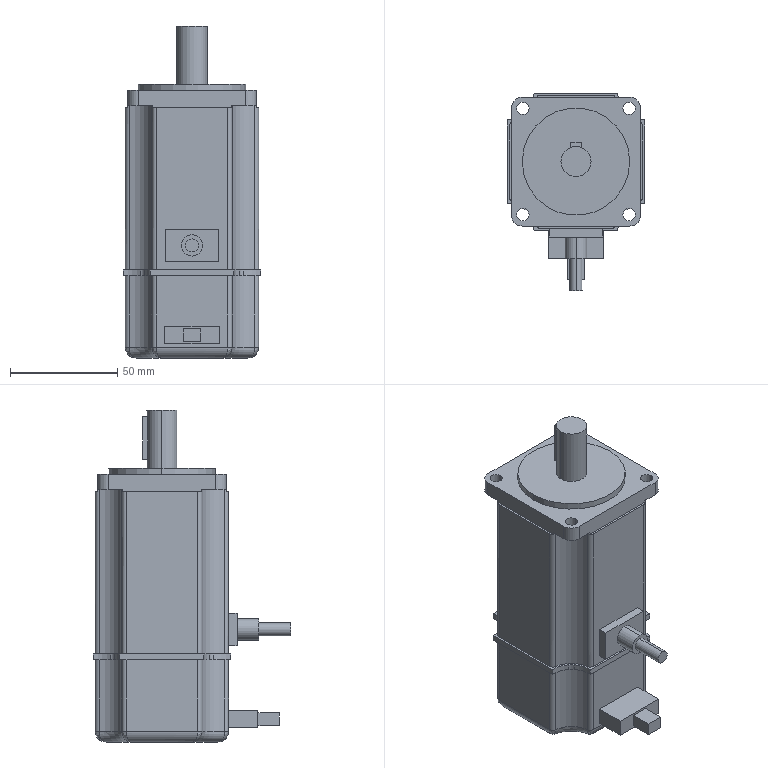Part | NX | features BREP 1 | 1 solid | 130 faces | box 64 x 92 x 154.5 mm | volume 181603 mm3 | cylinder 64 | plane 54 | spline 8 | torus 4 | commonest cylinder face diameters 4 x16 5.8 x12 23 x10 10 x8 25 x8 6 x2